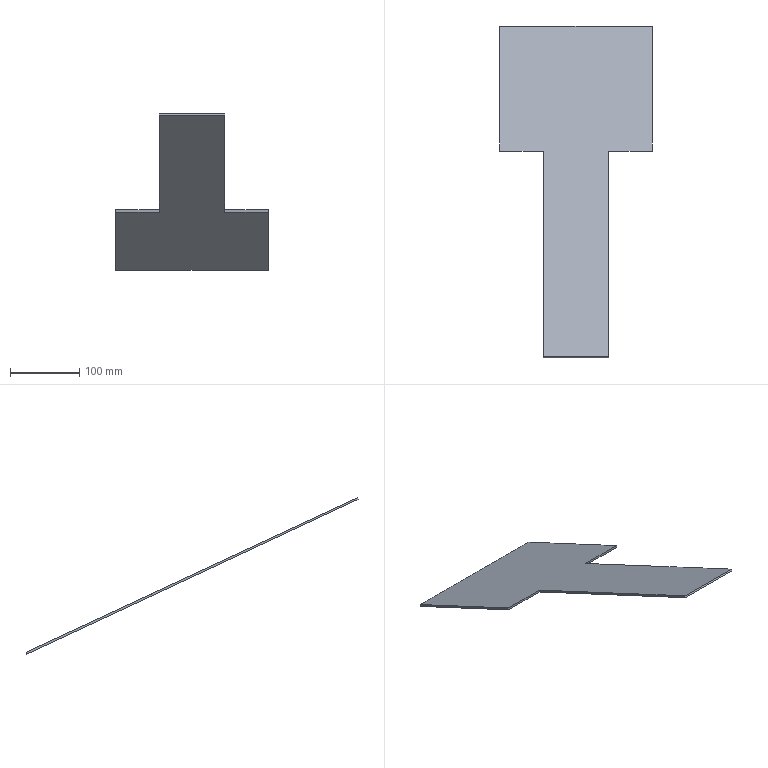Part | NX | features solid 2 | 1 solid | 10 faces | box 220 x 478 x 225.614 mm | volume 223608 mm3 | plane 10
STEP:
#1=CARTESIAN_POINT('',(-47.,360.,-255.65));
#2=VERTEX_POINT('',#1);
#3=CARTESIAN_POINT('',(-47.,360.,-258.96));
#4=VERTEX_POINT('',#3);
#5=CARTESIAN_POINT('',(-47.,360.,-300.));
#6=DIRECTION('',(0.,0.,-1.));
#7=VECTOR('',#6,1000.);
#8=LINE('',#5,#7);
#9=EDGE_CURVE('',#2,#4,#8,.T.);
#10=ORIENTED_EDGE('',*,*,#9,.F.);
#11=CARTESIAN_POINT('',(-110.,360.,-255.65));
#12=VERTEX_POINT('',#11);
#13=CARTESIAN_POINT('',(17.519,360.,-255.65));
#14=DIRECTION('',(1.,0.,0.));
#15=VECTOR('',#14,1000.);
#16=LINE('',#13,#15);
#17=EDGE_CURVE('',#12,#2,#16,.T.);
#18=ORIENTED_EDGE('',*,*,#17,.F.);
#19=CARTESIAN_POINT('',(-110.,360.,-258.96));
#20=VERTEX_POINT('',#19);
#21=CARTESIAN_POINT('',(-110.,360.,-130.));
#22=DIRECTION('',(0.,0.,-1.));
#23=VECTOR('',#22,1000.);
#24=LINE('',#21,#23);
#25=EDGE_CURVE('',#12,#20,#24,.T.);
#26=ORIENTED_EDGE('',*,*,#25,.T.);
#27=CARTESIAN_POINT('',(17.519,360.,-258.96));
#28=DIRECTION('',(1.,0.,0.));
#29=VECTOR('',#28,1000.);
#30=LINE('',#27,#29);
#31=EDGE_CURVE('',#20,#4,#30,.T.);
#32=ORIENTED_EDGE('',*,*,#31,.T.);
#33=EDGE_LOOP('',(#10,#18,#26,#32));
#34=FACE_BOUND('',#33,.T.);
#35=CARTESIAN_POINT('',(78.5,360.,-300.));
#36=DIRECTION('',(0.,1.,0.));
#37=DIRECTION('',(0.,0.,1.));
#38=AXIS2_PLACEMENT_3D('',#35,#36,#37);
#39=PLANE('',#38);
#40=ADVANCED_FACE('',(#34),#39,.F.);
#41=CARTESIAN_POINT('',(47.,360.,-258.96));
#42=VERTEX_POINT('',#41);
#43=CARTESIAN_POINT('',(47.,360.,-255.65));
#44=VERTEX_POINT('',#43);
#45=CARTESIAN_POINT('',(47.,360.,-300.));
#46=DIRECTION('',(0.,0.,1.));
#47=VECTOR('',#46,1000.);
#48=LINE('',#45,#47);
#49=EDGE_CURVE('',#42,#44,#48,.T.);
#50=ORIENTED_EDGE('',*,*,#49,.F.);
#51=CARTESIAN_POINT('',(110.,360.,-258.96));
#52=VERTEX_POINT('',#51);
#53=CARTESIAN_POINT('',(17.519,360.,-258.96));
#54=DIRECTION('',(1.,0.,0.));
#55=VECTOR('',#54,1000.);
#56=LINE('',#53,#55);
#57=EDGE_CURVE('',#42,#52,#56,.T.);
#58=ORIENTED_EDGE('',*,*,#57,.T.);
#59=CARTESIAN_POINT('',(110.,360.,-255.65));
#60=VERTEX_POINT('',#59);
#61=CARTESIAN_POINT('',(110.,360.,-130.));
#62=DIRECTION('',(0.,0.,1.));
#63=VECTOR('',#62,1000.);
#64=LINE('',#61,#63);
#65=EDGE_CURVE('',#52,#60,#64,.T.);
#66=ORIENTED_EDGE('',*,*,#65,.T.);
#67=CARTESIAN_POINT('',(17.519,360.,-255.65));
#68=DIRECTION('',(1.,0.,0.));
#69=VECTOR('',#68,1000.);
#70=LINE('',#67,#69);
#71=EDGE_CURVE('',#44,#60,#70,.T.);
#72=ORIENTED_EDGE('',*,*,#71,.F.);
#73=EDGE_LOOP('',(#50,#58,#66,#72));
#74=FACE_BOUND('',#73,.T.);
#75=CARTESIAN_POINT('',(78.5,360.,-300.));
#76=DIRECTION('',(0.,1.,0.));
#77=DIRECTION('',(0.,0.,1.));
#78=AXIS2_PLACEMENT_3D('',#75,#76,#77);
#79=PLANE('',#78);
#80=ADVANCED_FACE('',(#74),#79,.F.);
#81=CARTESIAN_POINT('',(-110.,540.,-339.585));
#82=VERTEX_POINT('',#81);
#83=CARTESIAN_POINT('',(-110.,540.,-342.895));
#84=VERTEX_POINT('',#83);
#85=CARTESIAN_POINT('',(-110.,540.,-130.));
#86=DIRECTION('',(0.,0.,1.));
#87=VECTOR('',#86,1000.);
#88=LINE('',#85,#87);
#89=EDGE_CURVE('',#82,#84,#88,.F.);
#90=ORIENTED_EDGE('',*,*,#89,.F.);
#91=CARTESIAN_POINT('',(110.,540.,-339.585));
#92=VERTEX_POINT('',#91);
#93=CARTESIAN_POINT('',(17.519,540.,-339.585));
#94=DIRECTION('',(-1.,0.,0.));
#95=VECTOR('',#94,1000.);
#96=LINE('',#93,#95);
#97=EDGE_CURVE('',#82,#92,#96,.F.);
#98=ORIENTED_EDGE('',*,*,#97,.T.);
#99=CARTESIAN_POINT('',(110.,540.,-342.895));
#100=VERTEX_POINT('',#99);
#101=CARTESIAN_POINT('',(110.,540.,-120.));
#102=DIRECTION('',(0.,0.,1.));
#103=VECTOR('',#102,1000.);
#104=LINE('',#101,#103);
#105=EDGE_CURVE('',#92,#100,#104,.F.);
#106=ORIENTED_EDGE('',*,*,#105,.T.);
#107=CARTESIAN_POINT('',(17.519,540.,-342.895));
#108=DIRECTION('',(-1.,0.,0.));
#109=VECTOR('',#108,1000.);
#110=LINE('',#107,#109);
#111=EDGE_CURVE('',#84,#100,#110,.F.);
#112=ORIENTED_EDGE('',*,*,#111,.F.);
#113=EDGE_LOOP('',(#90,#98,#106,#112));
#114=FACE_BOUND('',#113,.T.);
#115=CARTESIAN_POINT('',(1125.,540.,-120.));
#116=DIRECTION('',(0.,-1.,0.));
#117=DIRECTION('',(-1.,0.,0.));
#118=AXIS2_PLACEMENT_3D('',#115,#116,#117);
#119=PLANE('',#118);
#120=ADVANCED_FACE('',(#114),#119,.F.);
#121=CARTESIAN_POINT('',(-110.,63.268,-117.281));
#122=DIRECTION('',(0.,0.9063,-0.4226));
#123=VECTOR('',#122,1000.);
#124=LINE('',#121,#123);
#125=EDGE_CURVE('',#12,#82,#124,.T.);
#126=ORIENTED_EDGE('',*,*,#125,.F.);
#127=ORIENTED_EDGE('',*,*,#17,.T.);
#128=CARTESIAN_POINT('',(-47.,63.268,-117.281));
#129=VERTEX_POINT('',#128);
#130=CARTESIAN_POINT('',(-47.,63.268,-117.281));
#131=DIRECTION('',(0.,-0.9063,0.4226));
#132=VECTOR('',#131,1000.);
#133=LINE('',#130,#132);
#134=EDGE_CURVE('',#2,#129,#133,.T.);
#135=ORIENTED_EDGE('',*,*,#134,.T.);
#136=CARTESIAN_POINT('',(47.,63.268,-117.281));
#137=VERTEX_POINT('',#136);
#138=CARTESIAN_POINT('',(17.519,63.268,-117.281));
#139=DIRECTION('',(1.,0.,0.));
#140=VECTOR('',#139,1000.);
#141=LINE('',#138,#140);
#142=EDGE_CURVE('',#129,#137,#141,.T.);
#143=ORIENTED_EDGE('',*,*,#142,.T.);
#144=CARTESIAN_POINT('',(47.,63.268,-117.281));
#145=DIRECTION('',(0.,0.9063,-0.4226));
#146=VECTOR('',#145,1000.);
#147=LINE('',#144,#146);
#148=EDGE_CURVE('',#137,#44,#147,.T.);
#149=ORIENTED_EDGE('',*,*,#148,.T.);
#150=ORIENTED_EDGE('',*,*,#71,.T.);
#151=CARTESIAN_POINT('',(110.,67.098,-119.067));
#152=DIRECTION('',(0.,0.9063,-0.4226));
#153=VECTOR('',#152,1000.);
#154=LINE('',#151,#153);
#155=EDGE_CURVE('',#60,#92,#154,.T.);
#156=ORIENTED_EDGE('',*,*,#155,.T.);
#157=ORIENTED_EDGE('',*,*,#97,.F.);
#158=EDGE_LOOP('',(#126,#127,#135,#143,#149,#150,#156,#157));
#159=FACE_BOUND('',#158,.T.);
#160=CARTESIAN_POINT('',(17.519,63.268,-117.281));
#161=DIRECTION('',(0.,-0.4226,-0.9063));
#162=DIRECTION('',(0.,0.9063,-0.4226));
#163=AXIS2_PLACEMENT_3D('',#160,#161,#162);
#164=PLANE('',#163);
#165=ADVANCED_FACE('',(#159),#164,.F.);
#166=ORIENTED_EDGE('',*,*,#31,.F.);
#167=CARTESIAN_POINT('',(-110.,62.,-120.));
#168=DIRECTION('',(0.,0.9063,-0.4226));
#169=VECTOR('',#168,1000.);
#170=LINE('',#167,#169);
#171=EDGE_CURVE('',#20,#84,#170,.T.);
#172=ORIENTED_EDGE('',*,*,#171,.T.);
#173=ORIENTED_EDGE('',*,*,#111,.T.);
#174=CARTESIAN_POINT('',(110.,65.83,-121.786));
#175=DIRECTION('',(0.,0.9063,-0.4226));
#176=VECTOR('',#175,1000.);
#177=LINE('',#174,#176);
#178=EDGE_CURVE('',#52,#100,#177,.T.);
#179=ORIENTED_EDGE('',*,*,#178,.F.);
#180=ORIENTED_EDGE('',*,*,#57,.F.);
#181=CARTESIAN_POINT('',(47.,62.,-120.));
#182=VERTEX_POINT('',#181);
#183=CARTESIAN_POINT('',(47.,62.,-120.));
#184=DIRECTION('',(0.,0.9063,-0.4226));
#185=VECTOR('',#184,1000.);
#186=LINE('',#183,#185);
#187=EDGE_CURVE('',#182,#42,#186,.T.);
#188=ORIENTED_EDGE('',*,*,#187,.F.);
#189=CARTESIAN_POINT('',(-47.,62.,-120.));
#190=VERTEX_POINT('',#189);
#191=CARTESIAN_POINT('',(17.519,62.,-120.));
#192=DIRECTION('',(1.,0.,0.));
#193=VECTOR('',#192,1000.);
#194=LINE('',#191,#193);
#195=EDGE_CURVE('',#190,#182,#194,.T.);
#196=ORIENTED_EDGE('',*,*,#195,.F.);
#197=CARTESIAN_POINT('',(-47.,62.,-120.));
#198=DIRECTION('',(0.,-0.9063,0.4226));
#199=VECTOR('',#198,1000.);
#200=LINE('',#197,#199);
#201=EDGE_CURVE('',#4,#190,#200,.T.);
#202=ORIENTED_EDGE('',*,*,#201,.F.);
#203=EDGE_LOOP('',(#166,#172,#173,#179,#180,#188,#196,#202));
#204=FACE_BOUND('',#203,.T.);
#205=CARTESIAN_POINT('',(17.519,62.,-120.));
#206=DIRECTION('',(0.,-0.4226,-0.9063));
#207=DIRECTION('',(0.,0.9063,-0.4226));
#208=AXIS2_PLACEMENT_3D('',#205,#206,#207);
#209=PLANE('',#208);
#210=ADVANCED_FACE('',(#204),#209,.T.);
#211=ORIENTED_EDGE('',*,*,#65,.F.);
#212=ORIENTED_EDGE('',*,*,#178,.T.);
#213=ORIENTED_EDGE('',*,*,#105,.F.);
#214=ORIENTED_EDGE('',*,*,#155,.F.);
#215=EDGE_LOOP('',(#211,#212,#213,#214));
#216=FACE_BOUND('',#215,.T.);
#217=CARTESIAN_POINT('',(110.,62.,-130.));
#218=DIRECTION('',(1.,0.,0.));
#219=DIRECTION('',(0.,0.,1.));
#220=AXIS2_PLACEMENT_3D('',#217,#218,#219);
#221=PLANE('',#220);
#222=ADVANCED_FACE('',(#216),#221,.T.);
#223=ORIENTED_EDGE('',*,*,#25,.F.);
#224=ORIENTED_EDGE('',*,*,#125,.T.);
#225=ORIENTED_EDGE('',*,*,#89,.T.);
#226=ORIENTED_EDGE('',*,*,#171,.F.);
#227=EDGE_LOOP('',(#223,#224,#225,#226));
#228=FACE_BOUND('',#227,.T.);
#229=CARTESIAN_POINT('',(-110.,62.,-130.));
#230=DIRECTION('',(-1.,0.,0.));
#231=DIRECTION('',(0.,0.,1.));
#232=AXIS2_PLACEMENT_3D('',#229,#230,#231);
#233=PLANE('',#232);
#234=ADVANCED_FACE('',(#228),#233,.T.);
#235=CARTESIAN_POINT('',(-47.,62.,-120.));
#236=DIRECTION('',(0.,-0.4226,-0.9063));
#237=VECTOR('',#236,1000.);
#238=LINE('',#235,#237);
#239=EDGE_CURVE('',#190,#129,#238,.F.);
#240=ORIENTED_EDGE('',*,*,#239,.F.);
#241=ORIENTED_EDGE('',*,*,#195,.T.);
#242=CARTESIAN_POINT('',(47.,62.,-120.));
#243=DIRECTION('',(0.,0.4226,0.9063));
#244=VECTOR('',#243,1000.);
#245=LINE('',#242,#244);
#246=EDGE_CURVE('',#137,#182,#245,.F.);
#247=ORIENTED_EDGE('',*,*,#246,.F.);
#248=ORIENTED_EDGE('',*,*,#142,.F.);
#249=EDGE_LOOP('',(#240,#241,#247,#248));
#250=FACE_BOUND('',#249,.T.);
#251=CARTESIAN_POINT('',(17.519,62.,-120.));
#252=DIRECTION('',(0.,0.9063,-0.4226));
#253=DIRECTION('',(1.,0.,0.));
#254=AXIS2_PLACEMENT_3D('',#251,#252,#253);
#255=PLANE('',#254);
#256=ADVANCED_FACE('',(#250),#255,.F.);
#257=ORIENTED_EDGE('',*,*,#246,.T.);
#258=ORIENTED_EDGE('',*,*,#187,.T.);
#259=ORIENTED_EDGE('',*,*,#49,.T.);
#260=ORIENTED_EDGE('',*,*,#148,.F.);
#261=EDGE_LOOP('',(#257,#258,#259,#260));
#262=FACE_BOUND('',#261,.T.);
#263=CARTESIAN_POINT('',(47.,211.,-295.));
#264=DIRECTION('',(-1.,0.,0.));
#265=DIRECTION('',(0.,0.,1.));
#266=AXIS2_PLACEMENT_3D('',#263,#264,#265);
#267=PLANE('',#266);
#268=ADVANCED_FACE('',(#262),#267,.F.);
#269=ORIENTED_EDGE('',*,*,#239,.T.);
#270=ORIENTED_EDGE('',*,*,#134,.F.);
#271=ORIENTED_EDGE('',*,*,#9,.T.);
#272=ORIENTED_EDGE('',*,*,#201,.T.);
#273=EDGE_LOOP('',(#269,#270,#271,#272));
#274=FACE_BOUND('',#273,.T.);
#275=CARTESIAN_POINT('',(-47.,211.,-295.));
#276=DIRECTION('',(1.,0.,0.));
#277=DIRECTION('',(0.,0.,-1.));
#278=AXIS2_PLACEMENT_3D('',#275,#276,#277);
#279=PLANE('',#278);
#280=ADVANCED_FACE('',(#274),#279,.F.);
#281=CLOSED_SHELL('',(#40,#80,#120,#165,#210,#222,#234,#256,#268,#280));
#282=MANIFOLD_SOLID_BREP('',#281);
#283=(LENGTH_UNIT()NAMED_UNIT(*)SI_UNIT(.MILLI.,.METRE.));
#284=UNCERTAINTY_MEASURE_WITH_UNIT(LENGTH_MEASURE(0.00001),#283,'','');
#285=(NAMED_UNIT(*)PLANE_ANGLE_UNIT()SI_UNIT($,.RADIAN.));
#286=(NAMED_UNIT(*)SI_UNIT($,.STERADIAN.)SOLID_ANGLE_UNIT());
#287=(GEOMETRIC_REPRESENTATION_CONTEXT(3)GLOBAL_UNCERTAINTY_ASSIGNED_CONTEXT((#284))GLOBAL_UNIT_ASSIGNED_CONTEXT((#283,#285,#286))REPRESENTATION_CONTEXT('',''));
#288=ADVANCED_BREP_SHAPE_REPRESENTATION('',(#282),#287);